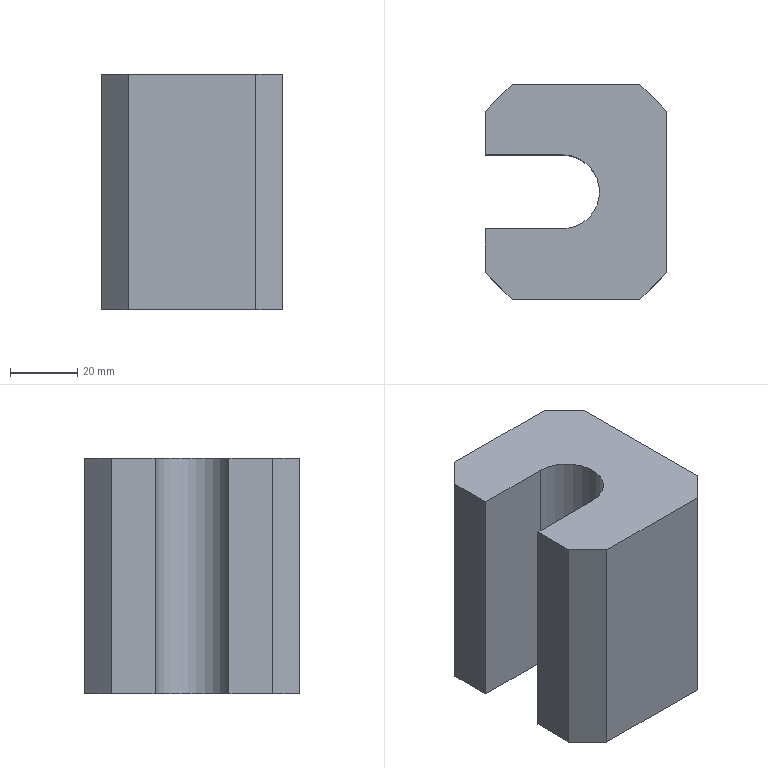Part | SolidWorks | features Extrusion 1 | 1 solid | 14 faces | box 54 x 64 x 70 mm | volume 184235 mm3 | plane 13 | cylinder 1 | commonest cylinder face diameters 22 x1
STEP:
#1=CARTESIAN_POINT('',(-54.,43.,0.));
#2=VERTEX_POINT('',#1);
#3=CARTESIAN_POINT('',(-31.,43.,0.));
#4=VERTEX_POINT('',#3);
#5=CARTESIAN_POINT('',(-54.,43.,0.));
#6=DIRECTION('',(1.,0.,0.));
#7=VECTOR('',#6,1000.);
#8=LINE('',#5,#7);
#9=EDGE_CURVE('',#2,#4,#8,.T.);
#10=ORIENTED_EDGE('',*,*,#9,.T.);
#11=CARTESIAN_POINT('',(-31.,43.,70.));
#12=VERTEX_POINT('',#11);
#13=CARTESIAN_POINT('',(-31.,43.,70.));
#14=DIRECTION('',(0.,0.,-1.));
#15=VECTOR('',#14,1000.);
#16=LINE('',#13,#15);
#17=EDGE_CURVE('',#12,#4,#16,.T.);
#18=ORIENTED_EDGE('',*,*,#17,.F.);
#19=CARTESIAN_POINT('',(-54.,43.,70.));
#20=VERTEX_POINT('',#19);
#21=CARTESIAN_POINT('',(-54.,43.,70.));
#22=DIRECTION('',(1.,0.,0.));
#23=VECTOR('',#22,1000.);
#24=LINE('',#21,#23);
#25=EDGE_CURVE('',#20,#12,#24,.T.);
#26=ORIENTED_EDGE('',*,*,#25,.F.);
#27=CARTESIAN_POINT('',(-54.,43.,70.));
#28=DIRECTION('',(0.,0.,-1.));
#29=VECTOR('',#28,1000.);
#30=LINE('',#27,#29);
#31=EDGE_CURVE('',#20,#2,#30,.T.);
#32=ORIENTED_EDGE('',*,*,#31,.T.);
#33=EDGE_LOOP('',(#10,#18,#26,#32));
#34=FACE_OUTER_BOUND('',#33,.T.);
#35=CARTESIAN_POINT('',(-54.,43.,70.));
#36=DIRECTION('',(0.,1.,0.));
#37=DIRECTION('',(0.,0.,1.));
#38=AXIS2_PLACEMENT_3D('',#35,#36,#37);
#39=PLANE('',#38);
#40=ADVANCED_FACE('',(#34),#39,.F.);
#41=CARTESIAN_POINT('',(-31.,21.,0.));
#42=VERTEX_POINT('',#41);
#43=CARTESIAN_POINT('',(-31.,32.,0.));
#44=DIRECTION('',(0.,0.,-1.));
#45=DIRECTION('',(1.,0.,0.));
#46=AXIS2_PLACEMENT_3D('',#43,#44,#45);
#47=CIRCLE('',#46,11.);
#48=EDGE_CURVE('',#4,#42,#47,.T.);
#49=ORIENTED_EDGE('',*,*,#48,.T.);
#50=CARTESIAN_POINT('',(-31.,21.,70.));
#51=VERTEX_POINT('',#50);
#52=CARTESIAN_POINT('',(-31.,21.,70.));
#53=DIRECTION('',(0.,0.,-1.));
#54=VECTOR('',#53,1000.);
#55=LINE('',#52,#54);
#56=EDGE_CURVE('',#51,#42,#55,.T.);
#57=ORIENTED_EDGE('',*,*,#56,.F.);
#58=CARTESIAN_POINT('',(-31.,32.,70.));
#59=DIRECTION('',(0.,0.,-1.));
#60=DIRECTION('',(1.,0.,0.));
#61=AXIS2_PLACEMENT_3D('',#58,#59,#60);
#62=CIRCLE('',#61,11.);
#63=EDGE_CURVE('',#12,#51,#62,.T.);
#64=ORIENTED_EDGE('',*,*,#63,.F.);
#65=ORIENTED_EDGE('',*,*,#17,.T.);
#66=EDGE_LOOP('',(#49,#57,#64,#65));
#67=FACE_OUTER_BOUND('',#66,.T.);
#68=CARTESIAN_POINT('',(-31.,32.,70.));
#69=DIRECTION('',(0.,0.,-1.));
#70=DIRECTION('',(-1.,0.,0.));
#71=AXIS2_PLACEMENT_3D('',#68,#69,#70);
#72=CYLINDRICAL_SURFACE('',#71,11.);
#73=ADVANCED_FACE('',(#67),#72,.F.);
#74=CARTESIAN_POINT('',(-54.,21.,0.));
#75=VERTEX_POINT('',#74);
#76=CARTESIAN_POINT('',(-54.,21.,0.));
#77=DIRECTION('',(-1.,0.,0.));
#78=VECTOR('',#77,1000.);
#79=LINE('',#76,#78);
#80=EDGE_CURVE('',#42,#75,#79,.T.);
#81=ORIENTED_EDGE('',*,*,#80,.T.);
#82=CARTESIAN_POINT('',(-54.,21.,70.));
#83=VERTEX_POINT('',#82);
#84=CARTESIAN_POINT('',(-54.,21.,70.));
#85=DIRECTION('',(0.,0.,-1.));
#86=VECTOR('',#85,1000.);
#87=LINE('',#84,#86);
#88=EDGE_CURVE('',#83,#75,#87,.T.);
#89=ORIENTED_EDGE('',*,*,#88,.F.);
#90=CARTESIAN_POINT('',(-54.,21.,70.));
#91=DIRECTION('',(-1.,0.,0.));
#92=VECTOR('',#91,1000.);
#93=LINE('',#90,#92);
#94=EDGE_CURVE('',#51,#83,#93,.T.);
#95=ORIENTED_EDGE('',*,*,#94,.F.);
#96=ORIENTED_EDGE('',*,*,#56,.T.);
#97=EDGE_LOOP('',(#81,#89,#95,#96));
#98=FACE_OUTER_BOUND('',#97,.T.);
#99=CARTESIAN_POINT('',(-54.,21.,70.));
#100=DIRECTION('',(0.,-1.,0.));
#101=DIRECTION('',(0.,0.,-1.));
#102=AXIS2_PLACEMENT_3D('',#99,#100,#101);
#103=PLANE('',#102);
#104=ADVANCED_FACE('',(#98),#103,.F.);
#105=CARTESIAN_POINT('',(-54.,8.,0.));
#106=VERTEX_POINT('',#105);
#107=CARTESIAN_POINT('',(-54.,8.,0.));
#108=DIRECTION('',(0.,-1.,0.));
#109=VECTOR('',#108,1000.);
#110=LINE('',#107,#109);
#111=EDGE_CURVE('',#75,#106,#110,.T.);
#112=ORIENTED_EDGE('',*,*,#111,.T.);
#113=CARTESIAN_POINT('',(-54.,8.,70.));
#114=VERTEX_POINT('',#113);
#115=CARTESIAN_POINT('',(-54.,8.,70.));
#116=DIRECTION('',(0.,0.,-1.));
#117=VECTOR('',#116,1000.);
#118=LINE('',#115,#117);
#119=EDGE_CURVE('',#114,#106,#118,.T.);
#120=ORIENTED_EDGE('',*,*,#119,.F.);
#121=CARTESIAN_POINT('',(-54.,8.,70.));
#122=DIRECTION('',(0.,-1.,0.));
#123=VECTOR('',#122,1000.);
#124=LINE('',#121,#123);
#125=EDGE_CURVE('',#83,#114,#124,.T.);
#126=ORIENTED_EDGE('',*,*,#125,.F.);
#127=ORIENTED_EDGE('',*,*,#88,.T.);
#128=EDGE_LOOP('',(#112,#120,#126,#127));
#129=FACE_OUTER_BOUND('',#128,.T.);
#130=CARTESIAN_POINT('',(-54.,8.,70.));
#131=DIRECTION('',(1.,0.,0.));
#132=DIRECTION('',(0.,0.,-1.));
#133=AXIS2_PLACEMENT_3D('',#130,#131,#132);
#134=PLANE('',#133);
#135=ADVANCED_FACE('',(#129),#134,.F.);
#136=CARTESIAN_POINT('',(-46.,0.,0.));
#137=VERTEX_POINT('',#136);
#138=CARTESIAN_POINT('',(-46.,0.,0.));
#139=DIRECTION('',(0.7071,-0.7071,0.));
#140=VECTOR('',#139,1000.);
#141=LINE('',#138,#140);
#142=EDGE_CURVE('',#106,#137,#141,.T.);
#143=ORIENTED_EDGE('',*,*,#142,.T.);
#144=CARTESIAN_POINT('',(-46.,0.,70.));
#145=VERTEX_POINT('',#144);
#146=CARTESIAN_POINT('',(-46.,0.,70.));
#147=DIRECTION('',(0.,0.,-1.));
#148=VECTOR('',#147,1000.);
#149=LINE('',#146,#148);
#150=EDGE_CURVE('',#145,#137,#149,.T.);
#151=ORIENTED_EDGE('',*,*,#150,.F.);
#152=CARTESIAN_POINT('',(-46.,0.,70.));
#153=DIRECTION('',(0.7071,-0.7071,0.));
#154=VECTOR('',#153,1000.);
#155=LINE('',#152,#154);
#156=EDGE_CURVE('',#114,#145,#155,.T.);
#157=ORIENTED_EDGE('',*,*,#156,.F.);
#158=ORIENTED_EDGE('',*,*,#119,.T.);
#159=EDGE_LOOP('',(#143,#151,#157,#158));
#160=FACE_OUTER_BOUND('',#159,.T.);
#161=CARTESIAN_POINT('',(-46.,0.,70.));
#162=DIRECTION('',(0.7071,0.7071,0.));
#163=DIRECTION('',(-0.7071,0.7071,0.));
#164=AXIS2_PLACEMENT_3D('',#161,#162,#163);
#165=PLANE('',#164);
#166=ADVANCED_FACE('',(#160),#165,.F.);
#167=CARTESIAN_POINT('',(-8.,0.,0.));
#168=VERTEX_POINT('',#167);
#169=CARTESIAN_POINT('',(-8.,0.,0.));
#170=DIRECTION('',(1.,0.,0.));
#171=VECTOR('',#170,1000.);
#172=LINE('',#169,#171);
#173=EDGE_CURVE('',#137,#168,#172,.T.);
#174=ORIENTED_EDGE('',*,*,#173,.T.);
#175=CARTESIAN_POINT('',(-8.,0.,70.));
#176=VERTEX_POINT('',#175);
#177=CARTESIAN_POINT('',(-8.,0.,70.));
#178=DIRECTION('',(0.,0.,-1.));
#179=VECTOR('',#178,1000.);
#180=LINE('',#177,#179);
#181=EDGE_CURVE('',#176,#168,#180,.T.);
#182=ORIENTED_EDGE('',*,*,#181,.F.);
#183=CARTESIAN_POINT('',(-8.,0.,70.));
#184=DIRECTION('',(1.,0.,0.));
#185=VECTOR('',#184,1000.);
#186=LINE('',#183,#185);
#187=EDGE_CURVE('',#145,#176,#186,.T.);
#188=ORIENTED_EDGE('',*,*,#187,.F.);
#189=ORIENTED_EDGE('',*,*,#150,.T.);
#190=EDGE_LOOP('',(#174,#182,#188,#189));
#191=FACE_OUTER_BOUND('',#190,.T.);
#192=CARTESIAN_POINT('',(-8.,0.,70.));
#193=DIRECTION('',(0.,1.,0.));
#194=DIRECTION('',(-1.,0.,0.));
#195=AXIS2_PLACEMENT_3D('',#192,#193,#194);
#196=PLANE('',#195);
#197=ADVANCED_FACE('',(#191),#196,.F.);
#198=CARTESIAN_POINT('',(0.,8.,0.));
#199=VERTEX_POINT('',#198);
#200=CARTESIAN_POINT('',(0.,8.,0.));
#201=DIRECTION('',(0.7071,0.7071,0.));
#202=VECTOR('',#201,1000.);
#203=LINE('',#200,#202);
#204=EDGE_CURVE('',#168,#199,#203,.T.);
#205=ORIENTED_EDGE('',*,*,#204,.T.);
#206=CARTESIAN_POINT('',(0.,8.,70.));
#207=VERTEX_POINT('',#206);
#208=CARTESIAN_POINT('',(0.,8.,70.));
#209=DIRECTION('',(0.,0.,-1.));
#210=VECTOR('',#209,1000.);
#211=LINE('',#208,#210);
#212=EDGE_CURVE('',#207,#199,#211,.T.);
#213=ORIENTED_EDGE('',*,*,#212,.F.);
#214=CARTESIAN_POINT('',(0.,8.,70.));
#215=DIRECTION('',(0.7071,0.7071,0.));
#216=VECTOR('',#215,1000.);
#217=LINE('',#214,#216);
#218=EDGE_CURVE('',#176,#207,#217,.T.);
#219=ORIENTED_EDGE('',*,*,#218,.F.);
#220=ORIENTED_EDGE('',*,*,#181,.T.);
#221=EDGE_LOOP('',(#205,#213,#219,#220));
#222=FACE_OUTER_BOUND('',#221,.T.);
#223=CARTESIAN_POINT('',(0.,8.,70.));
#224=DIRECTION('',(-0.7071,0.7071,0.));
#225=DIRECTION('',(-0.7071,-0.7071,0.));
#226=AXIS2_PLACEMENT_3D('',#223,#224,#225);
#227=PLANE('',#226);
#228=ADVANCED_FACE('',(#222),#227,.F.);
#229=CARTESIAN_POINT('',(0.,56.,0.));
#230=VERTEX_POINT('',#229);
#231=CARTESIAN_POINT('',(0.,8.,0.));
#232=DIRECTION('',(0.,1.,0.));
#233=VECTOR('',#232,1000.);
#234=LINE('',#231,#233);
#235=EDGE_CURVE('',#199,#230,#234,.T.);
#236=ORIENTED_EDGE('',*,*,#235,.T.);
#237=CARTESIAN_POINT('',(0.,56.,70.));
#238=VERTEX_POINT('',#237);
#239=CARTESIAN_POINT('',(0.,56.,70.));
#240=DIRECTION('',(0.,0.,-1.));
#241=VECTOR('',#240,1000.);
#242=LINE('',#239,#241);
#243=EDGE_CURVE('',#238,#230,#242,.T.);
#244=ORIENTED_EDGE('',*,*,#243,.F.);
#245=CARTESIAN_POINT('',(0.,8.,70.));
#246=DIRECTION('',(0.,1.,0.));
#247=VECTOR('',#246,1000.);
#248=LINE('',#245,#247);
#249=EDGE_CURVE('',#207,#238,#248,.T.);
#250=ORIENTED_EDGE('',*,*,#249,.F.);
#251=ORIENTED_EDGE('',*,*,#212,.T.);
#252=EDGE_LOOP('',(#236,#244,#250,#251));
#253=FACE_OUTER_BOUND('',#252,.T.);
#254=CARTESIAN_POINT('',(0.,8.,70.));
#255=DIRECTION('',(-1.,0.,0.));
#256=DIRECTION('',(0.,0.,1.));
#257=AXIS2_PLACEMENT_3D('',#254,#255,#256);
#258=PLANE('',#257);
#259=ADVANCED_FACE('',(#253),#258,.F.);
#260=CARTESIAN_POINT('',(-8.,64.,0.));
#261=VERTEX_POINT('',#260);
#262=CARTESIAN_POINT('',(0.,56.,0.));
#263=DIRECTION('',(-0.7071,0.7071,0.));
#264=VECTOR('',#263,1000.);
#265=LINE('',#262,#264);
#266=EDGE_CURVE('',#230,#261,#265,.T.);
#267=ORIENTED_EDGE('',*,*,#266,.T.);
#268=CARTESIAN_POINT('',(-8.,64.,70.));
#269=VERTEX_POINT('',#268);
#270=CARTESIAN_POINT('',(-8.,64.,70.));
#271=DIRECTION('',(0.,0.,-1.));
#272=VECTOR('',#271,1000.);
#273=LINE('',#270,#272);
#274=EDGE_CURVE('',#269,#261,#273,.T.);
#275=ORIENTED_EDGE('',*,*,#274,.F.);
#276=CARTESIAN_POINT('',(0.,56.,70.));
#277=DIRECTION('',(-0.7071,0.7071,0.));
#278=VECTOR('',#277,1000.);
#279=LINE('',#276,#278);
#280=EDGE_CURVE('',#238,#269,#279,.T.);
#281=ORIENTED_EDGE('',*,*,#280,.F.);
#282=ORIENTED_EDGE('',*,*,#243,.T.);
#283=EDGE_LOOP('',(#267,#275,#281,#282));
#284=FACE_OUTER_BOUND('',#283,.T.);
#285=CARTESIAN_POINT('',(0.,56.,70.));
#286=DIRECTION('',(-0.7071,-0.7071,0.));
#287=DIRECTION('',(0.7071,-0.7071,0.));
#288=AXIS2_PLACEMENT_3D('',#285,#286,#287);
#289=PLANE('',#288);
#290=ADVANCED_FACE('',(#284),#289,.F.);
#291=CARTESIAN_POINT('',(-46.,64.,0.));
#292=VERTEX_POINT('',#291);
#293=CARTESIAN_POINT('',(-8.,64.,0.));
#294=DIRECTION('',(-1.,0.,0.));
#295=VECTOR('',#294,1000.);
#296=LINE('',#293,#295);
#297=EDGE_CURVE('',#261,#292,#296,.T.);
#298=ORIENTED_EDGE('',*,*,#297,.T.);
#299=CARTESIAN_POINT('',(-46.,64.,70.));
#300=VERTEX_POINT('',#299);
#301=CARTESIAN_POINT('',(-46.,64.,70.));
#302=DIRECTION('',(0.,0.,-1.));
#303=VECTOR('',#302,1000.);
#304=LINE('',#301,#303);
#305=EDGE_CURVE('',#300,#292,#304,.T.);
#306=ORIENTED_EDGE('',*,*,#305,.F.);
#307=CARTESIAN_POINT('',(-8.,64.,70.));
#308=DIRECTION('',(-1.,0.,0.));
#309=VECTOR('',#308,1000.);
#310=LINE('',#307,#309);
#311=EDGE_CURVE('',#269,#300,#310,.T.);
#312=ORIENTED_EDGE('',*,*,#311,.F.);
#313=ORIENTED_EDGE('',*,*,#274,.T.);
#314=EDGE_LOOP('',(#298,#306,#312,#313));
#315=FACE_OUTER_BOUND('',#314,.T.);
#316=CARTESIAN_POINT('',(-8.,64.,70.));
#317=DIRECTION('',(0.,-1.,0.));
#318=DIRECTION('',(0.,0.,-1.));
#319=AXIS2_PLACEMENT_3D('',#316,#317,#318);
#320=PLANE('',#319);
#321=ADVANCED_FACE('',(#315),#320,.F.);
#322=CARTESIAN_POINT('',(-54.,56.,0.));
#323=VERTEX_POINT('',#322);
#324=CARTESIAN_POINT('',(-46.,64.,0.));
#325=DIRECTION('',(-0.7071,-0.7071,0.));
#326=VECTOR('',#325,1000.);
#327=LINE('',#324,#326);
#328=EDGE_CURVE('',#292,#323,#327,.T.);
#329=ORIENTED_EDGE('',*,*,#328,.T.);
#330=CARTESIAN_POINT('',(-54.,56.,70.));
#331=VERTEX_POINT('',#330);
#332=CARTESIAN_POINT('',(-54.,56.,70.));
#333=DIRECTION('',(0.,0.,-1.));
#334=VECTOR('',#333,1000.);
#335=LINE('',#332,#334);
#336=EDGE_CURVE('',#331,#323,#335,.T.);
#337=ORIENTED_EDGE('',*,*,#336,.F.);
#338=CARTESIAN_POINT('',(-46.,64.,70.));
#339=DIRECTION('',(-0.7071,-0.7071,0.));
#340=VECTOR('',#339,1000.);
#341=LINE('',#338,#340);
#342=EDGE_CURVE('',#300,#331,#341,.T.);
#343=ORIENTED_EDGE('',*,*,#342,.F.);
#344=ORIENTED_EDGE('',*,*,#305,.T.);
#345=EDGE_LOOP('',(#329,#337,#343,#344));
#346=FACE_OUTER_BOUND('',#345,.T.);
#347=CARTESIAN_POINT('',(-46.,64.,70.));
#348=DIRECTION('',(0.7071,-0.7071,0.));
#349=DIRECTION('',(0.7071,0.7071,0.));
#350=AXIS2_PLACEMENT_3D('',#347,#348,#349);
#351=PLANE('',#350);
#352=ADVANCED_FACE('',(#346),#351,.F.);
#353=CARTESIAN_POINT('',(-54.,56.,0.));
#354=DIRECTION('',(0.,-1.,0.));
#355=VECTOR('',#354,1000.);
#356=LINE('',#353,#355);
#357=EDGE_CURVE('',#323,#2,#356,.T.);
#358=ORIENTED_EDGE('',*,*,#357,.T.);
#359=ORIENTED_EDGE('',*,*,#31,.F.);
#360=CARTESIAN_POINT('',(-54.,56.,70.));
#361=DIRECTION('',(0.,-1.,0.));
#362=VECTOR('',#361,1000.);
#363=LINE('',#360,#362);
#364=EDGE_CURVE('',#331,#20,#363,.T.);
#365=ORIENTED_EDGE('',*,*,#364,.F.);
#366=ORIENTED_EDGE('',*,*,#336,.T.);
#367=EDGE_LOOP('',(#358,#359,#365,#366));
#368=FACE_OUTER_BOUND('',#367,.T.);
#369=CARTESIAN_POINT('',(-54.,56.,70.));
#370=DIRECTION('',(1.,0.,0.));
#371=DIRECTION('',(0.,0.,-1.));
#372=AXIS2_PLACEMENT_3D('',#369,#370,#371);
#373=PLANE('',#372);
#374=ADVANCED_FACE('',(#368),#373,.F.);
#375=ORIENTED_EDGE('',*,*,#25,.T.);
#376=ORIENTED_EDGE('',*,*,#63,.T.);
#377=ORIENTED_EDGE('',*,*,#94,.T.);
#378=ORIENTED_EDGE('',*,*,#125,.T.);
#379=ORIENTED_EDGE('',*,*,#156,.T.);
#380=ORIENTED_EDGE('',*,*,#187,.T.);
#381=ORIENTED_EDGE('',*,*,#218,.T.);
#382=ORIENTED_EDGE('',*,*,#249,.T.);
#383=ORIENTED_EDGE('',*,*,#280,.T.);
#384=ORIENTED_EDGE('',*,*,#311,.T.);
#385=ORIENTED_EDGE('',*,*,#342,.T.);
#386=ORIENTED_EDGE('',*,*,#364,.T.);
#387=EDGE_LOOP('',(#375,#376,#377,#378,#379,#380,#381,#382,#383,#384,#385,#386));
#388=FACE_OUTER_BOUND('',#387,.T.);
#389=CARTESIAN_POINT('',(-31.,32.,70.));
#390=DIRECTION('',(0.,0.,1.));
#391=DIRECTION('',(1.,0.,0.));
#392=AXIS2_PLACEMENT_3D('',#389,#390,#391);
#393=PLANE('',#392);
#394=ADVANCED_FACE('',(#388),#393,.T.);
#395=ORIENTED_EDGE('',*,*,#9,.F.);
#396=ORIENTED_EDGE('',*,*,#357,.F.);
#397=ORIENTED_EDGE('',*,*,#328,.F.);
#398=ORIENTED_EDGE('',*,*,#297,.F.);
#399=ORIENTED_EDGE('',*,*,#266,.F.);
#400=ORIENTED_EDGE('',*,*,#235,.F.);
#401=ORIENTED_EDGE('',*,*,#204,.F.);
#402=ORIENTED_EDGE('',*,*,#173,.F.);
#403=ORIENTED_EDGE('',*,*,#142,.F.);
#404=ORIENTED_EDGE('',*,*,#111,.F.);
#405=ORIENTED_EDGE('',*,*,#80,.F.);
#406=ORIENTED_EDGE('',*,*,#48,.F.);
#407=EDGE_LOOP('',(#395,#396,#397,#398,#399,#400,#401,#402,#403,#404,#405,#406));
#408=FACE_OUTER_BOUND('',#407,.T.);
#409=CARTESIAN_POINT('',(-31.,32.,0.));
#410=DIRECTION('',(0.,0.,1.));
#411=DIRECTION('',(1.,0.,0.));
#412=AXIS2_PLACEMENT_3D('',#409,#410,#411);
#413=PLANE('',#412);
#414=ADVANCED_FACE('',(#408),#413,.F.);
#415=CLOSED_SHELL('',(#40,#73,#104,#135,#166,#197,#228,#259,#290,#321,#352,#374,#394,#414));
#416=MANIFOLD_SOLID_BREP('',#415);
#417=CARTESIAN_POINT('',(0.,0.,0.));
#418=DIRECTION('',(0.,0.,1.));
#419=DIRECTION('',(1.,0.,0.));
#420=AXIS2_PLACEMENT_3D('',#417,#418,#419);
#421=(LENGTH_UNIT()NAMED_UNIT(*)SI_UNIT(.MILLI.,.METRE.));
#422=UNCERTAINTY_MEASURE_WITH_UNIT(LENGTH_MEASURE(0.00001),#421,'','');
#423=(NAMED_UNIT(*)PLANE_ANGLE_UNIT()SI_UNIT($,.RADIAN.));
#424=(NAMED_UNIT(*)SI_UNIT($,.STERADIAN.)SOLID_ANGLE_UNIT());
#425=(GEOMETRIC_REPRESENTATION_CONTEXT(3)GLOBAL_UNCERTAINTY_ASSIGNED_CONTEXT((#422))GLOBAL_UNIT_ASSIGNED_CONTEXT((#421,#423,#424))REPRESENTATION_CONTEXT('',''));
#426=ADVANCED_BREP_SHAPE_REPRESENTATION('',(#416,#420),#425);